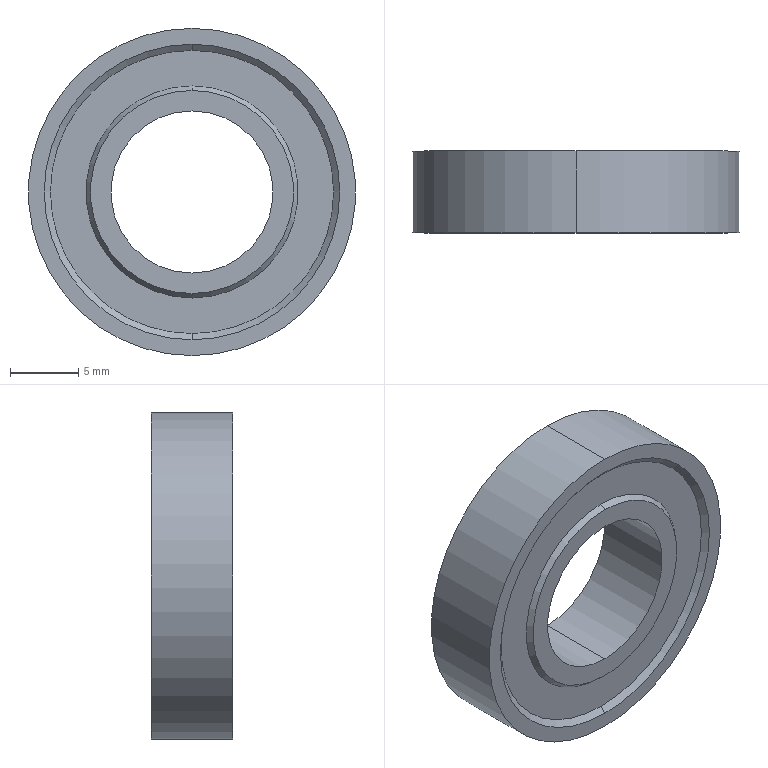Part | SolidWorks | features Revolution 1 | 1 solid | 18 faces | box 24 x 6 x 24 mm | volume 1915 mm3 | cone 8 | plane 6 | cylinder 4 | commonest cylinder face diameters 11.9 x2 24 x2
STEP:
#1=CARTESIAN_POINT('',(0.,-3.,-5.95));
#2=VERTEX_POINT('',#1);
#3=CARTESIAN_POINT('',(0.,-3.,5.95));
#4=VERTEX_POINT('',#3);
#5=CARTESIAN_POINT('',(0.,-3.,0.));
#6=DIRECTION('',(0.,1.,0.));
#7=DIRECTION('',(0.,0.,1.));
#8=AXIS2_PLACEMENT_3D('',#5,#6,#7);
#9=CIRCLE('',#8,5.95);
#10=EDGE_CURVE('',#2,#4,#9,.T.);
#11=ORIENTED_EDGE('',*,*,#10,.F.);
#12=CARTESIAN_POINT('',(0.,3.,-5.95));
#13=VERTEX_POINT('',#12);
#14=CARTESIAN_POINT('',(0.,19.601,-5.95));
#15=DIRECTION('',(0.,1.,0.));
#16=VECTOR('',#15,1000.);
#17=LINE('',#14,#16);
#18=EDGE_CURVE('',#2,#13,#17,.T.);
#19=ORIENTED_EDGE('',*,*,#18,.T.);
#20=CARTESIAN_POINT('',(0.,3.,5.95));
#21=VERTEX_POINT('',#20);
#22=CARTESIAN_POINT('',(0.,3.,0.));
#23=DIRECTION('',(0.,1.,0.));
#24=DIRECTION('',(0.,0.,1.));
#25=AXIS2_PLACEMENT_3D('',#22,#23,#24);
#26=CIRCLE('',#25,5.95);
#27=EDGE_CURVE('',#13,#21,#26,.T.);
#28=ORIENTED_EDGE('',*,*,#27,.T.);
#29=CARTESIAN_POINT('',(0.,19.601,5.95));
#30=DIRECTION('',(0.,1.,0.));
#31=VECTOR('',#30,1000.);
#32=LINE('',#29,#31);
#33=EDGE_CURVE('',#4,#21,#32,.T.);
#34=ORIENTED_EDGE('',*,*,#33,.F.);
#35=EDGE_LOOP('',(#11,#19,#28,#34));
#36=FACE_OUTER_BOUND('',#35,.T.);
#37=CARTESIAN_POINT('',(0.,19.601,0.));
#38=DIRECTION('',(0.,1.,0.));
#39=DIRECTION('',(0.,0.,1.));
#40=AXIS2_PLACEMENT_3D('',#37,#38,#39);
#41=CYLINDRICAL_SURFACE('',#40,5.95);
#42=ADVANCED_FACE('',(#36),#41,.F.);
#43=CARTESIAN_POINT('',(0.,-3.,7.45));
#44=VERTEX_POINT('',#43);
#45=CARTESIAN_POINT('',(0.,-3.,-7.45));
#46=VERTEX_POINT('',#45);
#47=CARTESIAN_POINT('',(0.,-3.,0.));
#48=DIRECTION('',(0.,1.,0.));
#49=DIRECTION('',(0.,0.,1.));
#50=AXIS2_PLACEMENT_3D('',#47,#48,#49);
#51=CIRCLE('',#50,7.45);
#52=EDGE_CURVE('',#44,#46,#51,.T.);
#53=ORIENTED_EDGE('',*,*,#52,.T.);
#54=CARTESIAN_POINT('',(0.,-2.614,-7.779));
#55=VERTEX_POINT('',#54);
#56=CARTESIAN_POINT('',(0.,-3.,-7.45));
#57=DIRECTION('',(0.,0.7606,-0.6492));
#58=VECTOR('',#57,1000.);
#59=LINE('',#56,#58);
#60=EDGE_CURVE('',#46,#55,#59,.T.);
#61=ORIENTED_EDGE('',*,*,#60,.T.);
#62=CARTESIAN_POINT('',(0.,-2.614,7.779));
#63=VERTEX_POINT('',#62);
#64=CARTESIAN_POINT('',(0.,-2.614,0.));
#65=DIRECTION('',(0.,1.,0.));
#66=DIRECTION('',(0.,0.,1.));
#67=AXIS2_PLACEMENT_3D('',#64,#65,#66);
#68=CIRCLE('',#67,7.779);
#69=EDGE_CURVE('',#63,#55,#68,.T.);
#70=ORIENTED_EDGE('',*,*,#69,.F.);
#71=CARTESIAN_POINT('',(0.,-3.,7.45));
#72=DIRECTION('',(0.,0.7606,0.6492));
#73=VECTOR('',#72,1000.);
#74=LINE('',#71,#73);
#75=EDGE_CURVE('',#44,#63,#74,.T.);
#76=ORIENTED_EDGE('',*,*,#75,.F.);
#77=EDGE_LOOP('',(#53,#61,#70,#76));
#78=FACE_OUTER_BOUND('',#77,.T.);
#79=CARTESIAN_POINT('',(0.,-3.,0.));
#80=DIRECTION('',(0.,1.,0.));
#81=DIRECTION('',(0.,0.,1.));
#82=AXIS2_PLACEMENT_3D('',#79,#80,#81);
#83=CONICAL_SURFACE('',#82,7.45,0.7065);
#84=ADVANCED_FACE('',(#78),#83,.T.);
#85=CARTESIAN_POINT('',(0.,-2.614,-10.386));
#86=VERTEX_POINT('',#85);
#87=CARTESIAN_POINT('',(0.,-2.614,10.386));
#88=VERTEX_POINT('',#87);
#89=CARTESIAN_POINT('',(0.,-2.614,0.));
#90=DIRECTION('',(0.,1.,0.));
#91=DIRECTION('',(0.,0.,1.));
#92=AXIS2_PLACEMENT_3D('',#89,#90,#91);
#93=CIRCLE('',#92,10.386);
#94=EDGE_CURVE('',#86,#88,#93,.T.);
#95=ORIENTED_EDGE('',*,*,#94,.T.);
#96=CARTESIAN_POINT('',(0.,-3.,10.838));
#97=VERTEX_POINT('',#96);
#98=CARTESIAN_POINT('',(0.,-2.614,10.386));
#99=DIRECTION('',(0.,-0.6492,0.7606));
#100=VECTOR('',#99,1000.);
#101=LINE('',#98,#100);
#102=EDGE_CURVE('',#88,#97,#101,.T.);
#103=ORIENTED_EDGE('',*,*,#102,.T.);
#104=CARTESIAN_POINT('',(0.,-3.,-10.838));
#105=VERTEX_POINT('',#104);
#106=CARTESIAN_POINT('',(0.,-3.,0.));
#107=DIRECTION('',(0.,1.,0.));
#108=DIRECTION('',(0.,0.,1.));
#109=AXIS2_PLACEMENT_3D('',#106,#107,#108);
#110=CIRCLE('',#109,10.838);
#111=EDGE_CURVE('',#105,#97,#110,.T.);
#112=ORIENTED_EDGE('',*,*,#111,.F.);
#113=CARTESIAN_POINT('',(0.,-2.614,-10.386));
#114=DIRECTION('',(0.,-0.6492,-0.7606));
#115=VECTOR('',#114,1000.);
#116=LINE('',#113,#115);
#117=EDGE_CURVE('',#86,#105,#116,.T.);
#118=ORIENTED_EDGE('',*,*,#117,.F.);
#119=EDGE_LOOP('',(#95,#103,#112,#118));
#120=FACE_OUTER_BOUND('',#119,.T.);
#121=CARTESIAN_POINT('',(0.,-2.614,0.));
#122=DIRECTION('',(0.,-1.,0.));
#123=DIRECTION('',(0.,0.,-1.));
#124=AXIS2_PLACEMENT_3D('',#121,#122,#123);
#125=CONICAL_SURFACE('',#124,10.386,0.8642);
#126=ADVANCED_FACE('',(#120),#125,.F.);
#127=CARTESIAN_POINT('',(0.,-3.,12.));
#128=VERTEX_POINT('',#127);
#129=CARTESIAN_POINT('',(0.,-3.,-12.));
#130=VERTEX_POINT('',#129);
#131=CARTESIAN_POINT('',(0.,-3.,0.));
#132=DIRECTION('',(0.,1.,0.));
#133=DIRECTION('',(0.,0.,1.));
#134=AXIS2_PLACEMENT_3D('',#131,#132,#133);
#135=CIRCLE('',#134,12.);
#136=EDGE_CURVE('',#128,#130,#135,.T.);
#137=ORIENTED_EDGE('',*,*,#136,.T.);
#138=CARTESIAN_POINT('',(0.,3.,-12.));
#139=VERTEX_POINT('',#138);
#140=CARTESIAN_POINT('',(0.,19.601,-12.));
#141=DIRECTION('',(0.,1.,0.));
#142=VECTOR('',#141,1000.);
#143=LINE('',#140,#142);
#144=EDGE_CURVE('',#130,#139,#143,.T.);
#145=ORIENTED_EDGE('',*,*,#144,.T.);
#146=CARTESIAN_POINT('',(0.,3.,12.));
#147=VERTEX_POINT('',#146);
#148=CARTESIAN_POINT('',(0.,3.,0.));
#149=DIRECTION('',(0.,1.,0.));
#150=DIRECTION('',(0.,0.,1.));
#151=AXIS2_PLACEMENT_3D('',#148,#149,#150);
#152=CIRCLE('',#151,12.);
#153=EDGE_CURVE('',#147,#139,#152,.T.);
#154=ORIENTED_EDGE('',*,*,#153,.F.);
#155=CARTESIAN_POINT('',(0.,19.601,12.));
#156=DIRECTION('',(0.,1.,0.));
#157=VECTOR('',#156,1000.);
#158=LINE('',#155,#157);
#159=EDGE_CURVE('',#128,#147,#158,.T.);
#160=ORIENTED_EDGE('',*,*,#159,.F.);
#161=EDGE_LOOP('',(#137,#145,#154,#160));
#162=FACE_OUTER_BOUND('',#161,.T.);
#163=CARTESIAN_POINT('',(0.,19.601,0.));
#164=DIRECTION('',(0.,1.,0.));
#165=DIRECTION('',(0.,0.,1.));
#166=AXIS2_PLACEMENT_3D('',#163,#164,#165);
#167=CYLINDRICAL_SURFACE('',#166,12.);
#168=ADVANCED_FACE('',(#162),#167,.T.);
#169=CARTESIAN_POINT('',(0.,2.614,-10.386));
#170=VERTEX_POINT('',#169);
#171=CARTESIAN_POINT('',(0.,2.614,10.386));
#172=VERTEX_POINT('',#171);
#173=CARTESIAN_POINT('',(0.,2.614,0.));
#174=DIRECTION('',(0.,1.,0.));
#175=DIRECTION('',(0.,0.,1.));
#176=AXIS2_PLACEMENT_3D('',#173,#174,#175);
#177=CIRCLE('',#176,10.386);
#178=EDGE_CURVE('',#170,#172,#177,.T.);
#179=ORIENTED_EDGE('',*,*,#178,.F.);
#180=CARTESIAN_POINT('',(0.,3.,-10.838));
#181=VERTEX_POINT('',#180);
#182=CARTESIAN_POINT('',(0.,3.,-10.838));
#183=DIRECTION('',(0.,0.6492,-0.7606));
#184=VECTOR('',#183,1000.);
#185=LINE('',#182,#184);
#186=EDGE_CURVE('',#170,#181,#185,.T.);
#187=ORIENTED_EDGE('',*,*,#186,.T.);
#188=CARTESIAN_POINT('',(0.,3.,10.838));
#189=VERTEX_POINT('',#188);
#190=CARTESIAN_POINT('',(0.,3.,0.));
#191=DIRECTION('',(0.,1.,0.));
#192=DIRECTION('',(0.,0.,1.));
#193=AXIS2_PLACEMENT_3D('',#190,#191,#192);
#194=CIRCLE('',#193,10.838);
#195=EDGE_CURVE('',#181,#189,#194,.T.);
#196=ORIENTED_EDGE('',*,*,#195,.T.);
#197=CARTESIAN_POINT('',(0.,3.,10.838));
#198=DIRECTION('',(0.,0.6492,0.7606));
#199=VECTOR('',#198,1000.);
#200=LINE('',#197,#199);
#201=EDGE_CURVE('',#172,#189,#200,.T.);
#202=ORIENTED_EDGE('',*,*,#201,.F.);
#203=EDGE_LOOP('',(#179,#187,#196,#202));
#204=FACE_OUTER_BOUND('',#203,.T.);
#205=CARTESIAN_POINT('',(0.,3.,0.));
#206=DIRECTION('',(0.,1.,0.));
#207=DIRECTION('',(0.,0.,1.));
#208=AXIS2_PLACEMENT_3D('',#205,#206,#207);
#209=CONICAL_SURFACE('',#208,10.838,0.8642);
#210=ADVANCED_FACE('',(#204),#209,.F.);
#211=CARTESIAN_POINT('',(0.,3.,7.45));
#212=VERTEX_POINT('',#211);
#213=CARTESIAN_POINT('',(0.,3.,-7.45));
#214=VERTEX_POINT('',#213);
#215=CARTESIAN_POINT('',(0.,3.,0.));
#216=DIRECTION('',(0.,1.,0.));
#217=DIRECTION('',(0.,0.,1.));
#218=AXIS2_PLACEMENT_3D('',#215,#216,#217);
#219=CIRCLE('',#218,7.45);
#220=EDGE_CURVE('',#212,#214,#219,.T.);
#221=ORIENTED_EDGE('',*,*,#220,.F.);
#222=CARTESIAN_POINT('',(0.,2.614,7.779));
#223=VERTEX_POINT('',#222);
#224=CARTESIAN_POINT('',(0.,2.614,7.779));
#225=DIRECTION('',(0.,-0.7606,0.6492));
#226=VECTOR('',#225,1000.);
#227=LINE('',#224,#226);
#228=EDGE_CURVE('',#212,#223,#227,.T.);
#229=ORIENTED_EDGE('',*,*,#228,.T.);
#230=CARTESIAN_POINT('',(0.,2.614,-7.779));
#231=VERTEX_POINT('',#230);
#232=CARTESIAN_POINT('',(0.,2.614,0.));
#233=DIRECTION('',(0.,1.,0.));
#234=DIRECTION('',(0.,0.,1.));
#235=AXIS2_PLACEMENT_3D('',#232,#233,#234);
#236=CIRCLE('',#235,7.779);
#237=EDGE_CURVE('',#223,#231,#236,.T.);
#238=ORIENTED_EDGE('',*,*,#237,.T.);
#239=CARTESIAN_POINT('',(0.,2.614,-7.779));
#240=DIRECTION('',(0.,-0.7606,-0.6492));
#241=VECTOR('',#240,1000.);
#242=LINE('',#239,#241);
#243=EDGE_CURVE('',#214,#231,#242,.T.);
#244=ORIENTED_EDGE('',*,*,#243,.F.);
#245=EDGE_LOOP('',(#221,#229,#238,#244));
#246=FACE_OUTER_BOUND('',#245,.T.);
#247=CARTESIAN_POINT('',(0.,2.614,0.));
#248=DIRECTION('',(0.,-1.,0.));
#249=DIRECTION('',(0.,0.,-1.));
#250=AXIS2_PLACEMENT_3D('',#247,#248,#249);
#251=CONICAL_SURFACE('',#250,7.779,0.7065);
#252=ADVANCED_FACE('',(#246),#251,.T.);
#253=CARTESIAN_POINT('',(0.,3.,0.));
#254=DIRECTION('',(0.,1.,0.));
#255=DIRECTION('',(0.,0.,1.));
#256=AXIS2_PLACEMENT_3D('',#253,#254,#255);
#257=CIRCLE('',#256,5.95);
#258=EDGE_CURVE('',#21,#13,#257,.T.);
#259=ORIENTED_EDGE('',*,*,#258,.F.);
#260=ORIENTED_EDGE('',*,*,#27,.F.);
#261=EDGE_LOOP('',(#259,#260));
#262=FACE_BOUND('',#261,.T.);
#263=CARTESIAN_POINT('',(0.,3.,0.));
#264=DIRECTION('',(0.,1.,0.));
#265=DIRECTION('',(0.,0.,1.));
#266=AXIS2_PLACEMENT_3D('',#263,#264,#265);
#267=CIRCLE('',#266,7.45);
#268=EDGE_CURVE('',#214,#212,#267,.T.);
#269=ORIENTED_EDGE('',*,*,#268,.T.);
#270=ORIENTED_EDGE('',*,*,#220,.T.);
#271=EDGE_LOOP('',(#269,#270));
#272=FACE_OUTER_BOUND('',#271,.T.);
#273=CARTESIAN_POINT('',(5.95,3.,0.));
#274=DIRECTION('',(0.,-1.,0.));
#275=DIRECTION('',(0.,0.,-1.));
#276=AXIS2_PLACEMENT_3D('',#273,#274,#275);
#277=PLANE('',#276);
#278=ADVANCED_FACE('',(#262,#272),#277,.F.);
#279=ORIENTED_EDGE('',*,*,#228,.F.);
#280=ORIENTED_EDGE('',*,*,#268,.F.);
#281=ORIENTED_EDGE('',*,*,#243,.T.);
#282=CARTESIAN_POINT('',(0.,2.614,0.));
#283=DIRECTION('',(0.,1.,0.));
#284=DIRECTION('',(0.,0.,1.));
#285=AXIS2_PLACEMENT_3D('',#282,#283,#284);
#286=CIRCLE('',#285,7.779);
#287=EDGE_CURVE('',#231,#223,#286,.T.);
#288=ORIENTED_EDGE('',*,*,#287,.T.);
#289=EDGE_LOOP('',(#279,#280,#281,#288));
#290=FACE_OUTER_BOUND('',#289,.T.);
#291=CARTESIAN_POINT('',(0.,2.614,0.));
#292=DIRECTION('',(0.,-1.,0.));
#293=DIRECTION('',(0.,0.,-1.));
#294=AXIS2_PLACEMENT_3D('',#291,#292,#293);
#295=CONICAL_SURFACE('',#294,7.779,0.7065);
#296=ADVANCED_FACE('',(#290),#295,.T.);
#297=ORIENTED_EDGE('',*,*,#287,.F.);
#298=ORIENTED_EDGE('',*,*,#237,.F.);
#299=EDGE_LOOP('',(#297,#298));
#300=FACE_BOUND('',#299,.T.);
#301=CARTESIAN_POINT('',(0.,2.614,0.));
#302=DIRECTION('',(0.,1.,0.));
#303=DIRECTION('',(0.,0.,1.));
#304=AXIS2_PLACEMENT_3D('',#301,#302,#303);
#305=CIRCLE('',#304,10.386);
#306=EDGE_CURVE('',#172,#170,#305,.T.);
#307=ORIENTED_EDGE('',*,*,#306,.T.);
#308=ORIENTED_EDGE('',*,*,#178,.T.);
#309=EDGE_LOOP('',(#307,#308));
#310=FACE_OUTER_BOUND('',#309,.T.);
#311=CARTESIAN_POINT('',(7.779,2.614,0.));
#312=DIRECTION('',(0.,-1.,0.));
#313=DIRECTION('',(0.,0.,-1.));
#314=AXIS2_PLACEMENT_3D('',#311,#312,#313);
#315=PLANE('',#314);
#316=ADVANCED_FACE('',(#300,#310),#315,.F.);
#317=ORIENTED_EDGE('',*,*,#186,.F.);
#318=ORIENTED_EDGE('',*,*,#306,.F.);
#319=ORIENTED_EDGE('',*,*,#201,.T.);
#320=CARTESIAN_POINT('',(0.,3.,0.));
#321=DIRECTION('',(0.,1.,0.));
#322=DIRECTION('',(0.,0.,1.));
#323=AXIS2_PLACEMENT_3D('',#320,#321,#322);
#324=CIRCLE('',#323,10.838);
#325=EDGE_CURVE('',#189,#181,#324,.T.);
#326=ORIENTED_EDGE('',*,*,#325,.T.);
#327=EDGE_LOOP('',(#317,#318,#319,#326));
#328=FACE_OUTER_BOUND('',#327,.T.);
#329=CARTESIAN_POINT('',(0.,3.,0.));
#330=DIRECTION('',(0.,1.,0.));
#331=DIRECTION('',(0.,0.,1.));
#332=AXIS2_PLACEMENT_3D('',#329,#330,#331);
#333=CONICAL_SURFACE('',#332,10.838,0.8642);
#334=ADVANCED_FACE('',(#328),#333,.F.);
#335=ORIENTED_EDGE('',*,*,#325,.F.);
#336=ORIENTED_EDGE('',*,*,#195,.F.);
#337=EDGE_LOOP('',(#335,#336));
#338=FACE_BOUND('',#337,.T.);
#339=ORIENTED_EDGE('',*,*,#153,.T.);
#340=CARTESIAN_POINT('',(0.,3.,0.));
#341=DIRECTION('',(0.,1.,0.));
#342=DIRECTION('',(0.,0.,1.));
#343=AXIS2_PLACEMENT_3D('',#340,#341,#342);
#344=CIRCLE('',#343,12.);
#345=EDGE_CURVE('',#139,#147,#344,.T.);
#346=ORIENTED_EDGE('',*,*,#345,.T.);
#347=EDGE_LOOP('',(#339,#346));
#348=FACE_OUTER_BOUND('',#347,.T.);
#349=CARTESIAN_POINT('',(10.838,3.,0.));
#350=DIRECTION('',(0.,-1.,0.));
#351=DIRECTION('',(0.,0.,-1.));
#352=AXIS2_PLACEMENT_3D('',#349,#350,#351);
#353=PLANE('',#352);
#354=ADVANCED_FACE('',(#338,#348),#353,.F.);
#355=ORIENTED_EDGE('',*,*,#144,.F.);
#356=CARTESIAN_POINT('',(0.,-3.,0.));
#357=DIRECTION('',(0.,1.,0.));
#358=DIRECTION('',(0.,0.,1.));
#359=AXIS2_PLACEMENT_3D('',#356,#357,#358);
#360=CIRCLE('',#359,12.);
#361=EDGE_CURVE('',#130,#128,#360,.T.);
#362=ORIENTED_EDGE('',*,*,#361,.T.);
#363=ORIENTED_EDGE('',*,*,#159,.T.);
#364=ORIENTED_EDGE('',*,*,#345,.F.);
#365=EDGE_LOOP('',(#355,#362,#363,#364));
#366=FACE_OUTER_BOUND('',#365,.T.);
#367=CARTESIAN_POINT('',(0.,19.601,0.));
#368=DIRECTION('',(0.,1.,0.));
#369=DIRECTION('',(0.,0.,1.));
#370=AXIS2_PLACEMENT_3D('',#367,#368,#369);
#371=CYLINDRICAL_SURFACE('',#370,12.);
#372=ADVANCED_FACE('',(#366),#371,.T.);
#373=ORIENTED_EDGE('',*,*,#136,.F.);
#374=ORIENTED_EDGE('',*,*,#361,.F.);
#375=EDGE_LOOP('',(#373,#374));
#376=FACE_OUTER_BOUND('',#375,.T.);
#377=ORIENTED_EDGE('',*,*,#111,.T.);
#378=CARTESIAN_POINT('',(0.,-3.,0.));
#379=DIRECTION('',(0.,1.,0.));
#380=DIRECTION('',(0.,0.,1.));
#381=AXIS2_PLACEMENT_3D('',#378,#379,#380);
#382=CIRCLE('',#381,10.838);
#383=EDGE_CURVE('',#97,#105,#382,.T.);
#384=ORIENTED_EDGE('',*,*,#383,.T.);
#385=EDGE_LOOP('',(#377,#384));
#386=FACE_BOUND('',#385,.T.);
#387=CARTESIAN_POINT('',(10.838,-3.,0.));
#388=DIRECTION('',(0.,1.,0.));
#389=DIRECTION('',(0.,0.,1.));
#390=AXIS2_PLACEMENT_3D('',#387,#388,#389);
#391=PLANE('',#390);
#392=ADVANCED_FACE('',(#376,#386),#391,.F.);
#393=ORIENTED_EDGE('',*,*,#102,.F.);
#394=CARTESIAN_POINT('',(0.,-2.614,0.));
#395=DIRECTION('',(0.,1.,0.));
#396=DIRECTION('',(0.,0.,1.));
#397=AXIS2_PLACEMENT_3D('',#394,#395,#396);
#398=CIRCLE('',#397,10.386);
#399=EDGE_CURVE('',#88,#86,#398,.T.);
#400=ORIENTED_EDGE('',*,*,#399,.T.);
#401=ORIENTED_EDGE('',*,*,#117,.T.);
#402=ORIENTED_EDGE('',*,*,#383,.F.);
#403=EDGE_LOOP('',(#393,#400,#401,#402));
#404=FACE_OUTER_BOUND('',#403,.T.);
#405=CARTESIAN_POINT('',(0.,-2.614,0.));
#406=DIRECTION('',(0.,-1.,0.));
#407=DIRECTION('',(0.,0.,-1.));
#408=AXIS2_PLACEMENT_3D('',#405,#406,#407);
#409=CONICAL_SURFACE('',#408,10.386,0.8642);
#410=ADVANCED_FACE('',(#404),#409,.F.);
#411=ORIENTED_EDGE('',*,*,#94,.F.);
#412=ORIENTED_EDGE('',*,*,#399,.F.);
#413=EDGE_LOOP('',(#411,#412));
#414=FACE_OUTER_BOUND('',#413,.T.);
#415=ORIENTED_EDGE('',*,*,#69,.T.);
#416=CARTESIAN_POINT('',(0.,-2.614,0.));
#417=DIRECTION('',(0.,1.,0.));
#418=DIRECTION('',(0.,0.,1.));
#419=AXIS2_PLACEMENT_3D('',#416,#417,#418);
#420=CIRCLE('',#419,7.779);
#421=EDGE_CURVE('',#55,#63,#420,.T.);
#422=ORIENTED_EDGE('',*,*,#421,.T.);
#423=EDGE_LOOP('',(#415,#422));
#424=FACE_BOUND('',#423,.T.);
#425=CARTESIAN_POINT('',(7.779,-2.614,0.));
#426=DIRECTION('',(0.,1.,0.));
#427=DIRECTION('',(0.,0.,1.));
#428=AXIS2_PLACEMENT_3D('',#425,#426,#427);
#429=PLANE('',#428);
#430=ADVANCED_FACE('',(#414,#424),#429,.F.);
#431=ORIENTED_EDGE('',*,*,#60,.F.);
#432=CARTESIAN_POINT('',(0.,-3.,0.));
#433=DIRECTION('',(0.,1.,0.));
#434=DIRECTION('',(0.,0.,1.));
#435=AXIS2_PLACEMENT_3D('',#432,#433,#434);
#436=CIRCLE('',#435,7.45);
#437=EDGE_CURVE('',#46,#44,#436,.T.);
#438=ORIENTED_EDGE('',*,*,#437,.T.);
#439=ORIENTED_EDGE('',*,*,#75,.T.);
#440=ORIENTED_EDGE('',*,*,#421,.F.);
#441=EDGE_LOOP('',(#431,#438,#439,#440));
#442=FACE_OUTER_BOUND('',#441,.T.);
#443=CARTESIAN_POINT('',(0.,-3.,0.));
#444=DIRECTION('',(0.,1.,0.));
#445=DIRECTION('',(0.,0.,1.));
#446=AXIS2_PLACEMENT_3D('',#443,#444,#445);
#447=CONICAL_SURFACE('',#446,7.45,0.7065);
#448=ADVANCED_FACE('',(#442),#447,.T.);
#449=ORIENTED_EDGE('',*,*,#52,.F.);
#450=ORIENTED_EDGE('',*,*,#437,.F.);
#451=EDGE_LOOP('',(#449,#450));
#452=FACE_OUTER_BOUND('',#451,.T.);
#453=CARTESIAN_POINT('',(0.,-3.,0.));
#454=DIRECTION('',(0.,1.,0.));
#455=DIRECTION('',(0.,0.,1.));
#456=AXIS2_PLACEMENT_3D('',#453,#454,#455);
#457=CIRCLE('',#456,5.95);
#458=EDGE_CURVE('',#4,#2,#457,.T.);
#459=ORIENTED_EDGE('',*,*,#458,.T.);
#460=ORIENTED_EDGE('',*,*,#10,.T.);
#461=EDGE_LOOP('',(#459,#460));
#462=FACE_BOUND('',#461,.T.);
#463=CARTESIAN_POINT('',(5.95,-3.,0.));
#464=DIRECTION('',(0.,1.,0.));
#465=DIRECTION('',(0.,0.,1.));
#466=AXIS2_PLACEMENT_3D('',#463,#464,#465);
#467=PLANE('',#466);
#468=ADVANCED_FACE('',(#452,#462),#467,.F.);
#469=ORIENTED_EDGE('',*,*,#18,.F.);
#470=ORIENTED_EDGE('',*,*,#458,.F.);
#471=ORIENTED_EDGE('',*,*,#33,.T.);
#472=ORIENTED_EDGE('',*,*,#258,.T.);
#473=EDGE_LOOP('',(#469,#470,#471,#472));
#474=FACE_OUTER_BOUND('',#473,.T.);
#475=CARTESIAN_POINT('',(0.,19.601,0.));
#476=DIRECTION('',(0.,1.,0.));
#477=DIRECTION('',(0.,0.,1.));
#478=AXIS2_PLACEMENT_3D('',#475,#476,#477);
#479=CYLINDRICAL_SURFACE('',#478,5.95);
#480=ADVANCED_FACE('',(#474),#479,.F.);
#481=CLOSED_SHELL('',(#42,#84,#126,#168,#210,#252,#278,#296,#316,#334,#354,#372,#392,#410,#430,#448,#468,#480));
#482=MANIFOLD_SOLID_BREP('',#481);
#483=CARTESIAN_POINT('',(0.,0.,0.));
#484=DIRECTION('',(0.,0.,1.));
#485=DIRECTION('',(1.,0.,0.));
#486=AXIS2_PLACEMENT_3D('',#483,#484,#485);
#487=(LENGTH_UNIT()NAMED_UNIT(*)SI_UNIT(.MILLI.,.METRE.));
#488=UNCERTAINTY_MEASURE_WITH_UNIT(LENGTH_MEASURE(0.00001),#487,'','');
#489=(NAMED_UNIT(*)PLANE_ANGLE_UNIT()SI_UNIT($,.RADIAN.));
#490=(NAMED_UNIT(*)SI_UNIT($,.STERADIAN.)SOLID_ANGLE_UNIT());
#491=(GEOMETRIC_REPRESENTATION_CONTEXT(3)GLOBAL_UNCERTAINTY_ASSIGNED_CONTEXT((#488))GLOBAL_UNIT_ASSIGNED_CONTEXT((#487,#489,#490))REPRESENTATION_CONTEXT('',''));
#492=ADVANCED_BREP_SHAPE_REPRESENTATION('',(#482,#486),#491);